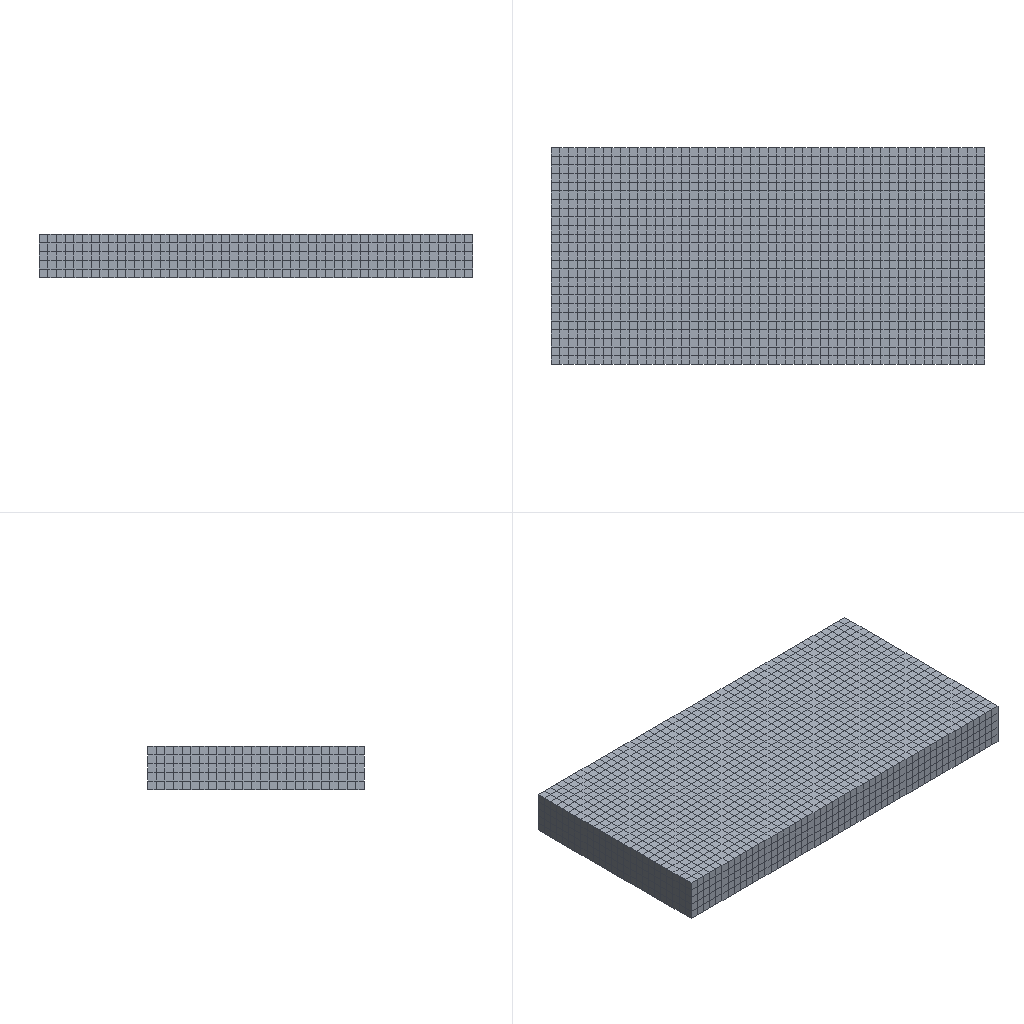Simulation study | abaqus
Abaqus input file, long lists of numbers shortened:
*Heading
** Job name: deck-2 Model name: Model-1-Copy
** Generated by: Abaqus/CAE 2024
*Preprint, echo=NO, model=NO, history=NO, contact=NO
**
** PARTS
**
*Part, name=Part-1
*Node
      1,           0.,         -25.,           5.
      2,           0.,         -24.,           5.
** (7954 more lines like these left out)
*Element, type=C3D8R
   1,  157,  158,  184,  183,    1,    2,   28,   27
   2,  158,  159,  185,  184,    2,    3,   29,   28
** (6248 more lines like these left out)
*Nset, nset=Set-1, generate
    1,  7956,     1
*Elset, elset=Set-1, generate
    1,  6250,     1
** Section: Section-1
*Solid Section, elset=Set-1, material=Material-1
,
*End Part
**
*Part, name=tool
*Node
      1,           5.,         10.5,           2.
      2,           5.,   3.762,           2.
** (472 more lines like these left out)
*Element, type=R3D4
 1,   1,   9, 109,  40
 2,   9,  10, 110, 109
** (470 more lines like these left out)
*Node
    475,           5.,         10.5,           1.
*Nset, nset=tool-RefPt_, internal
475,
*Elset, elset=tool, generate
   1,  472,    1
*End Part
**
**
** ASSEMBLY
**
*Assembly, name=Assembly
**
*Instance, name=Part-1-1, part=Part-1
*End Instance
**
*Instance, name=tool-1, part=tool
         50.,        -11.5,           0.
         50.,        -11.5,           0., 51.,        -11.5,           0., 90.
*End Instance
**
*Instance, name=tool-1-lin-2-1, part=tool
         50.,         -5.5,           0.
         50.,         -5.5,           0., 51.,         -5.5,           0., 90.
*End Instance
**
*Instance, name=tool-1-lin-2-1-1, part=tool
         50.,        -17.5,           0.
         50.,        -17.5,           0., 51.,        -17.5,           0., 90.
*End Instance
**
*Nset, nset=Set-1, instance=Part-1-1
  131,  132,  133,  134,  135,  136,  137,  138,  139,  140,  141,  142,  143,  144,  145,  146
  147,  148,  149,  150,  151,  152,  153,  154,  155,  156,  287,  288,  289,  290,  291,  292
** (81 more lines like these left out)
*Elset, elset=Set-1, instance=Part-1-1
  101,  102,  103,  104,  105,  106,  107,  108,  109,  110,  111,  112,  113,  114,  115,  116
  117,  118,  119,  120,  121,  122,  123,  124,  125,  226,  227,  228,  229,  230,  231,  232
** (77 more lines like these left out)
*Nset, nset=Set-3, instance=tool-1-lin-2-1-1
 475,
*Nset, nset=Set-4, instance=tool-1
 475,
*Nset, nset=Set-5, instance=tool-1-lin-2-1
 475,
*Nset, nset=s_Set-2, instance=Part-1-1, generate
    1,  7956,     1
*Elset, elset=s_Set-2, instance=Part-1-1, generate
    1,  6250,     1
*Elset, elset=_m_Surf-1_SPOS, internal, instance=tool-1-lin-2-1-1, generate
   1,  472,    1
*Surface, type=ELEMENT, name=m_Surf-1
_m_Surf-1_SPOS, SPOS
*Elset, elset=_m_Surf-2_SPOS, internal, instance=tool-1, generate
   1,  472,    1
*Surface, type=ELEMENT, name=m_Surf-2
_m_Surf-2_SPOS, SPOS
*Elset, elset=_m_Surf-3_SPOS, internal, instance=tool-1-lin-2-1, generate
   1,  472,    1
*Surface, type=ELEMENT, name=m_Surf-3
_m_Surf-3_SPOS, SPOS
*Surface, type=NODE, name=s_Set-2_CNS_, internal
s_Set-2, 1.
*Rigid Body, ref node=tool-1.tool-RefPt_, elset=tool-1.tool
*Rigid Body, ref node=tool-1-lin-2-1.tool-RefPt_, elset=tool-1-lin-2-1.tool
*Rigid Body, ref node=tool-1-lin-2-1-1.tool-RefPt_, elset=tool-1-lin-2-1-1.tool
*End Assembly
**
** MATERIALS
**
*Material, name=Material-1
*Damage Initiation, criterion=SHEAR
 0.1,0.,0.
*Damage Evolution, type=DISPLACEMENT
 1e-05,
*Density
 2.8e-09,
*Elastic
72000., 0.3
*Plastic
200.,0.
**
** INTERACTION PROPERTIES
**
*Surface Interaction, name=IntProp-1
*Friction
 0.2,
*Surface Behavior, pressure-overclosure=HARD
** ----------------------------------------------------------------
**
** STEP: Step-1
**
*Step, name=Step-1, nlgeom=YES
*Dynamic, Explicit
, 0.01
*Bulk Viscosity
0.06, 1.2
** Mass Scaling: Semi-Automatic
**               Whole Model
*Fixed Mass Scaling, factor=500.
**
** BOUNDARY CONDITIONS
**
** Name: BC-fix Type: Symmetry/Antisymmetry/Encastre
*Boundary
Set-1, ENCASTRE
** Name: BC-v1 Type: Velocity/Angular velocity
*Boundary, type=VELOCITY
Set-3, 1, 1, -5600.
Set-3, 2, 2
Set-3, 3, 3
Set-3, 4, 4
Set-3, 5, 5
Set-3, 6, 6
** Name: BC-v2 Type: Velocity/Angular velocity
*Boundary, type=VELOCITY
Set-4, 1, 1
Set-4, 2, 2
Set-4, 3, 3
Set-4, 4, 4
Set-4, 5, 5
Set-4, 6, 6
** Name: BC-v3 Type: Velocity/Angular velocity
*Boundary, type=VELOCITY
Set-5, 1, 1
Set-5, 2, 2
Set-5, 3, 3
Set-5, 4, 4
Set-5, 5, 5
Set-5, 6, 6
**
** INTERACTIONS
**
** Interaction: Int-1
*Contact Pair, interaction=IntProp-1, mechanical constraint=KINEMATIC, cpset=Int-1
m_Surf-1, s_Set-2_CNS_
** Interaction: Int-1-Copy
*Contact Pair, interaction=IntProp-1, mechanical constraint=KINEMATIC, cpset=Int-1-Copy
m_Surf-2, s_Set-2_CNS_
** Interaction: Int-1-Copy2
*Contact Pair, interaction=IntProp-1, mechanical constraint=KINEMATIC, cpset=Int-1-Copy2
m_Surf-3, s_Set-2_CNS_
**
** OUTPUT REQUESTS
**
*Restart, write, number interval=1, time marks=NO
**
** FIELD OUTPUT: F-Output-1
**
*Output, field, number interval=40
*Node Output
A, CF, RF, RM, RT, U, V
*Element Output, directions=YES
E, EVF, LE, MISES, MISESMAX, PE, PEEQ, PEEQVAVG, PEVAVG, S, STATUS, SVAVG
*Contact Output
CDISP, CSTRESS
**
** HISTORY OUTPUT: H-Output-1
**
*Output, history, time interval=2e-07
*Node Output, nset=Set-1
RF1, RF2, RF3
*End Step
** ----------------------------------------------------------------
**
** STEP: Step-2
**
*Step, name=Step-2, nlgeom=YES
*Dynamic, Explicit
, 0.01
*Bulk Viscosity
0.06, 1.2
** Mass Scaling: Semi-Automatic
**               Whole Model
*Fixed Mass Scaling, factor=500.
**
** BOUNDARY CONDITIONS
**
** Name: BC-v1 Type: Velocity/Angular velocity
*Boundary, type=VELOCITY
Set-3, 1, 1
** Name: BC-v2 Type: Velocity/Angular velocity
*Boundary, type=VELOCITY
Set-4, 1, 1, -5600.
**
** OUTPUT REQUESTS
**
*Restart, write, number interval=1, time marks=NO
**
** FIELD OUTPUT: F-Output-1
**
*Output, field, number interval=40
*Node Output
A, CF, RF, RM, RT, U, V
*Element Output, directions=YES
E, EVF, LE, MISES, MISESMAX, PE, PEEQ, PEEQVAVG, PEVAVG, S, STATUS, SVAVG
*Contact Output
CDISP, CSTRESS
**
** HISTORY OUTPUT: H-Output-2
**
*Output, history, time interval=2e-07
*Node Output, nset=Set-3
RF1, RF2, RF3
*End Step
** ----------------------------------------------------------------
**
** STEP: Step-3
**
*Step, name=Step-3, nlgeom=YES
*Dynamic, Explicit
, 0.01
*Bulk Viscosity
0.06, 1.2
** Mass Scaling: Semi-Automatic
**               Whole Model
*Fixed Mass Scaling, factor=500.
**
** BOUNDARY CONDITIONS
**
** Name: BC-v2 Type: Velocity/Angular velocity
*Boundary, type=VELOCITY
Set-4, 1, 1
** Name: BC-v3 Type: Velocity/Angular velocity
*Boundary, type=VELOCITY
Set-5, 1, 1, -5600.
**
** OUTPUT REQUESTS
**
*Restart, write, number interval=1, time marks=NO
**
** FIELD OUTPUT: F-Output-1
**
*Output, field, number interval=40
*Node Output
A, CF, RF, RM, RT, U, V
*Element Output, directions=YES
E, EVF, LE, MISES, MISESMAX, PE, PEEQ, PEEQVAVG, PEVAVG, S, STATUS, SVAVG
*Contact Output
CDISP, CSTRESS
**
** HISTORY OUTPUT: H-Output-3
**
*Output, history, time interval=2e-07
*Node Output, nset=Set-5
RF1, RF2, RF3
*End Step